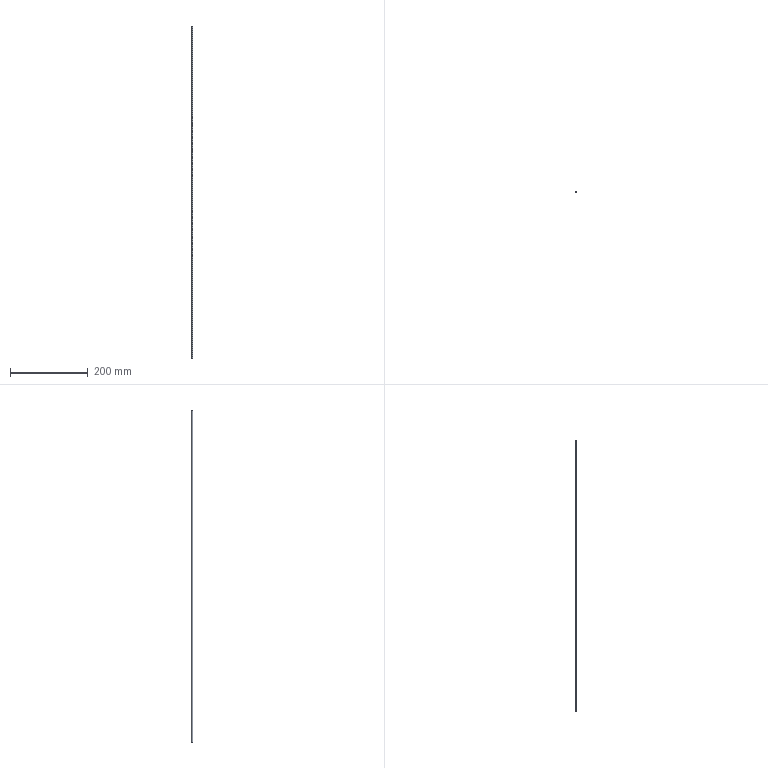Part | STEP file | PZ-G51EP-Part-1-3 | 1 solid | 4 faces | box 3 x 3 x 855 mm | volume 6044 mm3 | cylinder 2 | plane 2 | commonest cylinder face diameters 3 x2
STEP:
#1=CARTESIAN_POINT('',(0.,5.5,855.));
#2=VERTEX_POINT('',#1);
#3=CARTESIAN_POINT('',(0.,2.5,855.));
#4=VERTEX_POINT('',#3);
#5=CARTESIAN_POINT('',(0.,4.,855.));
#6=DIRECTION('',(0.,0.,-1.));
#7=DIRECTION('',(0.,1.,0.));
#8=AXIS2_PLACEMENT_3D('',#5,#6,#7);
#9=CIRCLE('',#8,1.5);
#10=EDGE_CURVE('',#2,#4,#9,.T.);
#11=ORIENTED_EDGE('',*,*,#10,.T.);
#12=CARTESIAN_POINT('',(0.,2.5,0.));
#13=VERTEX_POINT('',#12);
#14=CARTESIAN_POINT('',(0.,2.5,855.));
#15=DIRECTION('',(0.,0.,-1.));
#16=VECTOR('',#15,1000.);
#17=LINE('',#14,#16);
#18=EDGE_CURVE('',#4,#13,#17,.T.);
#19=ORIENTED_EDGE('',*,*,#18,.T.);
#20=CARTESIAN_POINT('',(0.,5.5,0.));
#21=VERTEX_POINT('',#20);
#22=CARTESIAN_POINT('',(0.,4.,0.));
#23=DIRECTION('',(0.,0.,1.));
#24=DIRECTION('',(0.,-1.,0.));
#25=AXIS2_PLACEMENT_3D('',#22,#23,#24);
#26=CIRCLE('',#25,1.5);
#27=EDGE_CURVE('',#13,#21,#26,.T.);
#28=ORIENTED_EDGE('',*,*,#27,.T.);
#29=CARTESIAN_POINT('',(0.,5.5,855.));
#30=DIRECTION('',(0.,0.,-1.));
#31=VECTOR('',#30,1000.);
#32=LINE('',#29,#31);
#33=EDGE_CURVE('',#2,#21,#32,.T.);
#34=ORIENTED_EDGE('',*,*,#33,.F.);
#35=EDGE_LOOP('',(#11,#19,#28,#34));
#36=FACE_OUTER_BOUND('',#35,.T.);
#37=CARTESIAN_POINT('',(0.,4.,855.));
#38=DIRECTION('',(0.,0.,-1.));
#39=DIRECTION('',(0.,1.,0.));
#40=AXIS2_PLACEMENT_3D('',#37,#38,#39);
#41=CYLINDRICAL_SURFACE('',#40,1.5);
#42=ADVANCED_FACE('',(#36),#41,.T.);
#43=CARTESIAN_POINT('',(0.,4.,0.));
#44=DIRECTION('',(0.,0.,1.));
#45=DIRECTION('',(0.,-1.,0.));
#46=AXIS2_PLACEMENT_3D('',#43,#44,#45);
#47=CIRCLE('',#46,1.5);
#48=EDGE_CURVE('',#21,#13,#47,.T.);
#49=ORIENTED_EDGE('',*,*,#48,.F.);
#50=ORIENTED_EDGE('',*,*,#27,.F.);
#51=EDGE_LOOP('',(#49,#50));
#52=FACE_OUTER_BOUND('',#51,.T.);
#53=CARTESIAN_POINT('',(0.,4.,0.));
#54=DIRECTION('',(0.,0.,-1.));
#55=DIRECTION('',(0.,1.,0.));
#56=AXIS2_PLACEMENT_3D('',#53,#54,#55);
#57=PLANE('',#56);
#58=ADVANCED_FACE('',(#52),#57,.T.);
#59=ORIENTED_EDGE('',*,*,#10,.F.);
#60=CARTESIAN_POINT('',(0.,4.,855.));
#61=DIRECTION('',(0.,0.,-1.));
#62=DIRECTION('',(0.,1.,0.));
#63=AXIS2_PLACEMENT_3D('',#60,#61,#62);
#64=CIRCLE('',#63,1.5);
#65=EDGE_CURVE('',#4,#2,#64,.T.);
#66=ORIENTED_EDGE('',*,*,#65,.F.);
#67=EDGE_LOOP('',(#59,#66));
#68=FACE_OUTER_BOUND('',#67,.T.);
#69=CARTESIAN_POINT('',(0.,4.,855.));
#70=DIRECTION('',(0.,0.,1.));
#71=DIRECTION('',(0.,-1.,0.));
#72=AXIS2_PLACEMENT_3D('',#69,#70,#71);
#73=PLANE('',#72);
#74=ADVANCED_FACE('',(#68),#73,.T.);
#75=ORIENTED_EDGE('',*,*,#18,.F.);
#76=ORIENTED_EDGE('',*,*,#65,.T.);
#77=ORIENTED_EDGE('',*,*,#33,.T.);
#78=ORIENTED_EDGE('',*,*,#48,.T.);
#79=EDGE_LOOP('',(#75,#76,#77,#78));
#80=FACE_OUTER_BOUND('',#79,.T.);
#81=CARTESIAN_POINT('',(0.,4.,855.));
#82=DIRECTION('',(0.,0.,-1.));
#83=DIRECTION('',(0.,1.,0.));
#84=AXIS2_PLACEMENT_3D('',#81,#82,#83);
#85=CYLINDRICAL_SURFACE('',#84,1.5);
#86=ADVANCED_FACE('',(#80),#85,.T.);
#87=CLOSED_SHELL('',(#42,#58,#74,#86));
#88=MANIFOLD_SOLID_BREP('',#87);
#89=CARTESIAN_POINT('',(0.,0.,0.));
#90=DIRECTION('',(0.,0.,1.));
#91=DIRECTION('',(1.,0.,0.));
#92=AXIS2_PLACEMENT_3D('',#89,#90,#91);
#93=(LENGTH_UNIT()NAMED_UNIT(*)SI_UNIT(.MILLI.,.METRE.));
#94=UNCERTAINTY_MEASURE_WITH_UNIT(LENGTH_MEASURE(0.00001),#93,'','');
#95=(NAMED_UNIT(*)PLANE_ANGLE_UNIT()SI_UNIT($,.RADIAN.));
#96=(NAMED_UNIT(*)SI_UNIT($,.STERADIAN.)SOLID_ANGLE_UNIT());
#97=(GEOMETRIC_REPRESENTATION_CONTEXT(3)GLOBAL_UNCERTAINTY_ASSIGNED_CONTEXT((#94))GLOBAL_UNIT_ASSIGNED_CONTEXT((#93,#95,#96))REPRESENTATION_CONTEXT('',''));
#98=ADVANCED_BREP_SHAPE_REPRESENTATION('',(#88,#92),#97);